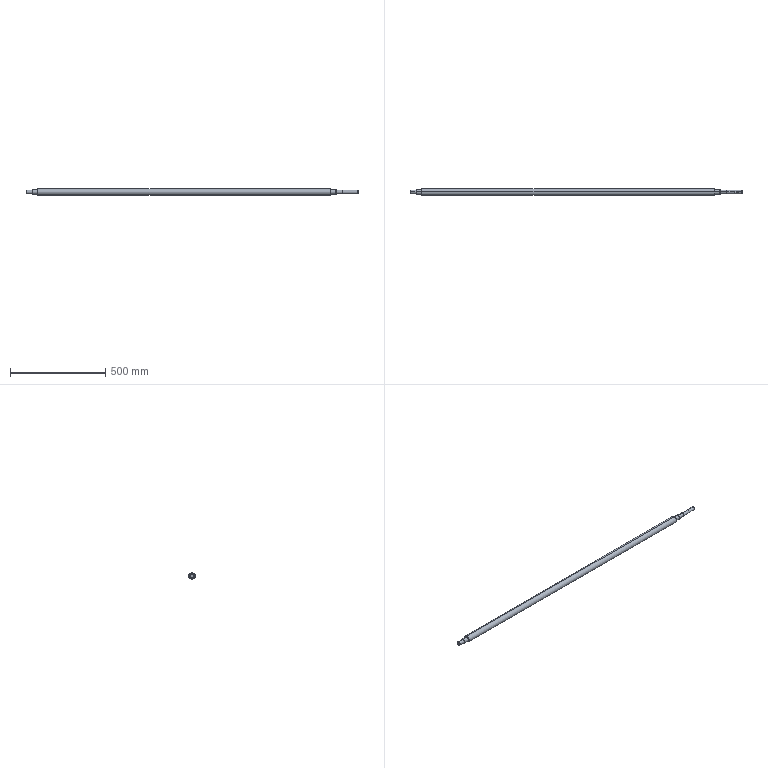Part | STEP file | Microwave Drying Flat Conveyor-CN2500x400-107-101 | 1 solid | 49 faces | box 1746 x 35 x 35 mm | volume 1552118 mm3 | cylinder 20 | cone 14 | plane 11 | torus 4 | commonest cylinder face diameters 0.4 x4 6 x4 20 x4 25 x4 18 x2 35 x2
STEP:
#1=CARTESIAN_POINT('',(-831.3,0.,9.));
#2=VERTEX_POINT('',#1);
#3=CARTESIAN_POINT('',(-831.3,0.,-9.));
#4=VERTEX_POINT('',#3);
#5=CARTESIAN_POINT('',(-831.3,0.,0.));
#6=DIRECTION('',(-1.,0.,0.));
#7=DIRECTION('',(0.,0.,-1.));
#8=AXIS2_PLACEMENT_3D('',#5,#6,#7);
#9=CIRCLE('',#8,9.);
#10=EDGE_CURVE('',#2,#4,#9,.T.);
#11=ORIENTED_EDGE('',*,*,#10,.F.);
#12=CARTESIAN_POINT('',(-830.3,0.,10.));
#13=VERTEX_POINT('',#12);
#14=CARTESIAN_POINT('',(-831.3,0.,9.));
#15=DIRECTION('',(0.7071,0.,0.7071));
#16=VECTOR('',#15,1000.);
#17=LINE('',#14,#16);
#18=EDGE_CURVE('',#2,#13,#17,.T.);
#19=ORIENTED_EDGE('',*,*,#18,.T.);
#20=CARTESIAN_POINT('',(-830.3,0.,-10.));
#21=VERTEX_POINT('',#20);
#22=CARTESIAN_POINT('',(-830.3,0.,0.));
#23=DIRECTION('',(1.,0.,0.));
#24=DIRECTION('',(0.,0.,-1.));
#25=AXIS2_PLACEMENT_3D('',#22,#23,#24);
#26=CIRCLE('',#25,10.);
#27=EDGE_CURVE('',#21,#13,#26,.T.);
#28=ORIENTED_EDGE('',*,*,#27,.F.);
#29=CARTESIAN_POINT('',(-831.3,0.,-9.));
#30=DIRECTION('',(0.7071,0.,-0.7071));
#31=VECTOR('',#30,1000.);
#32=LINE('',#29,#31);
#33=EDGE_CURVE('',#4,#21,#32,.T.);
#34=ORIENTED_EDGE('',*,*,#33,.F.);
#35=EDGE_LOOP('',(#11,#19,#28,#34));
#36=FACE_OUTER_BOUND('',#35,.T.);
#37=CARTESIAN_POINT('',(-831.3,0.,0.));
#38=DIRECTION('',(1.,0.,0.));
#39=DIRECTION('',(0.,0.,-1.));
#40=AXIS2_PLACEMENT_3D('',#37,#38,#39);
#41=CONICAL_SURFACE('',#40,9.,0.7854);
#42=ADVANCED_FACE('',(#36),#41,.T.);
#43=CARTESIAN_POINT('',(-799.3,0.,11.5));
#44=VERTEX_POINT('',#43);
#45=CARTESIAN_POINT('',(-799.3,0.,-11.5));
#46=VERTEX_POINT('',#45);
#47=CARTESIAN_POINT('',(-799.3,0.,0.));
#48=DIRECTION('',(-1.,0.,0.));
#49=DIRECTION('',(0.,0.,-1.));
#50=AXIS2_PLACEMENT_3D('',#47,#48,#49);
#51=CIRCLE('',#50,11.5);
#52=EDGE_CURVE('',#44,#46,#51,.T.);
#53=ORIENTED_EDGE('',*,*,#52,.F.);
#54=CARTESIAN_POINT('',(-798.3,0.,12.5));
#55=VERTEX_POINT('',#54);
#56=CARTESIAN_POINT('',(-799.3,0.,11.5));
#57=DIRECTION('',(0.7071,0.,0.7071));
#58=VECTOR('',#57,1000.);
#59=LINE('',#56,#58);
#60=EDGE_CURVE('',#44,#55,#59,.T.);
#61=ORIENTED_EDGE('',*,*,#60,.T.);
#62=CARTESIAN_POINT('',(-798.3,0.,-12.5));
#63=VERTEX_POINT('',#62);
#64=CARTESIAN_POINT('',(-798.3,0.,0.));
#65=DIRECTION('',(1.,0.,0.));
#66=DIRECTION('',(0.,0.,-1.));
#67=AXIS2_PLACEMENT_3D('',#64,#65,#66);
#68=CIRCLE('',#67,12.5);
#69=EDGE_CURVE('',#63,#55,#68,.T.);
#70=ORIENTED_EDGE('',*,*,#69,.F.);
#71=CARTESIAN_POINT('',(-799.3,0.,-11.5));
#72=DIRECTION('',(0.7071,0.,-0.7071));
#73=VECTOR('',#72,1000.);
#74=LINE('',#71,#73);
#75=EDGE_CURVE('',#46,#63,#74,.T.);
#76=ORIENTED_EDGE('',*,*,#75,.F.);
#77=EDGE_LOOP('',(#53,#61,#70,#76));
#78=FACE_OUTER_BOUND('',#77,.T.);
#79=CARTESIAN_POINT('',(-799.3,0.,0.));
#80=DIRECTION('',(1.,0.,0.));
#81=DIRECTION('',(0.,0.,-1.));
#82=AXIS2_PLACEMENT_3D('',#79,#80,#81);
#83=CONICAL_SURFACE('',#82,11.5,0.7854);
#84=ADVANCED_FACE('',(#78),#83,.T.);
#85=CARTESIAN_POINT('',(-771.,0.,16.5));
#86=VERTEX_POINT('',#85);
#87=CARTESIAN_POINT('',(-771.,0.,-16.5));
#88=VERTEX_POINT('',#87);
#89=CARTESIAN_POINT('',(-771.,0.,0.));
#90=DIRECTION('',(-1.,0.,0.));
#91=DIRECTION('',(0.,0.,-1.));
#92=AXIS2_PLACEMENT_3D('',#89,#90,#91);
#93=CIRCLE('',#92,16.5);
#94=EDGE_CURVE('',#86,#88,#93,.T.);
#95=ORIENTED_EDGE('',*,*,#94,.F.);
#96=CARTESIAN_POINT('',(-770.,0.,17.5));
#97=VERTEX_POINT('',#96);
#98=CARTESIAN_POINT('',(-771.,0.,16.5));
#99=DIRECTION('',(0.7071,0.,0.7071));
#100=VECTOR('',#99,1000.);
#101=LINE('',#98,#100);
#102=EDGE_CURVE('',#86,#97,#101,.T.);
#103=ORIENTED_EDGE('',*,*,#102,.T.);
#104=CARTESIAN_POINT('',(-770.,0.,-17.5));
#105=VERTEX_POINT('',#104);
#106=CARTESIAN_POINT('',(-770.,0.,0.));
#107=DIRECTION('',(1.,0.,0.));
#108=DIRECTION('',(0.,0.,-1.));
#109=AXIS2_PLACEMENT_3D('',#106,#107,#108);
#110=CIRCLE('',#109,17.5);
#111=EDGE_CURVE('',#105,#97,#110,.T.);
#112=ORIENTED_EDGE('',*,*,#111,.F.);
#113=CARTESIAN_POINT('',(-771.,0.,-16.5));
#114=DIRECTION('',(0.7071,0.,-0.7071));
#115=VECTOR('',#114,1000.);
#116=LINE('',#113,#115);
#117=EDGE_CURVE('',#88,#105,#116,.T.);
#118=ORIENTED_EDGE('',*,*,#117,.F.);
#119=EDGE_LOOP('',(#95,#103,#112,#118));
#120=FACE_OUTER_BOUND('',#119,.T.);
#121=CARTESIAN_POINT('',(-771.,0.,0.));
#122=DIRECTION('',(1.,0.,0.));
#123=DIRECTION('',(0.,0.,-1.));
#124=AXIS2_PLACEMENT_3D('',#121,#122,#123);
#125=CONICAL_SURFACE('',#124,16.5,0.7854);
#126=ADVANCED_FACE('',(#120),#125,.T.);
#127=CARTESIAN_POINT('',(771.,0.,-16.5));
#128=VERTEX_POINT('',#127);
#129=CARTESIAN_POINT('',(771.,0.,16.5));
#130=VERTEX_POINT('',#129);
#131=CARTESIAN_POINT('',(771.,0.,0.));
#132=DIRECTION('',(1.,0.,0.));
#133=DIRECTION('',(0.,0.,1.));
#134=AXIS2_PLACEMENT_3D('',#131,#132,#133);
#135=CIRCLE('',#134,16.5);
#136=EDGE_CURVE('',#128,#130,#135,.T.);
#137=ORIENTED_EDGE('',*,*,#136,.F.);
#138=CARTESIAN_POINT('',(770.,0.,-17.5));
#139=VERTEX_POINT('',#138);
#140=CARTESIAN_POINT('',(770.,0.,-17.5));
#141=DIRECTION('',(-0.7071,0.,-0.7071));
#142=VECTOR('',#141,1000.);
#143=LINE('',#140,#142);
#144=EDGE_CURVE('',#128,#139,#143,.T.);
#145=ORIENTED_EDGE('',*,*,#144,.T.);
#146=CARTESIAN_POINT('',(770.,0.,17.5));
#147=VERTEX_POINT('',#146);
#148=CARTESIAN_POINT('',(770.,0.,0.));
#149=DIRECTION('',(-1.,0.,0.));
#150=DIRECTION('',(0.,0.,1.));
#151=AXIS2_PLACEMENT_3D('',#148,#149,#150);
#152=CIRCLE('',#151,17.5);
#153=EDGE_CURVE('',#147,#139,#152,.T.);
#154=ORIENTED_EDGE('',*,*,#153,.F.);
#155=CARTESIAN_POINT('',(770.,0.,17.5));
#156=DIRECTION('',(-0.7071,0.,0.7071));
#157=VECTOR('',#156,1000.);
#158=LINE('',#155,#157);
#159=EDGE_CURVE('',#130,#147,#158,.T.);
#160=ORIENTED_EDGE('',*,*,#159,.F.);
#161=EDGE_LOOP('',(#137,#145,#154,#160));
#162=FACE_OUTER_BOUND('',#161,.T.);
#163=CARTESIAN_POINT('',(770.,0.,0.));
#164=DIRECTION('',(-1.,0.,0.));
#165=DIRECTION('',(0.,0.,1.));
#166=AXIS2_PLACEMENT_3D('',#163,#164,#165);
#167=CONICAL_SURFACE('',#166,17.5,0.7854);
#168=ADVANCED_FACE('',(#162),#167,.T.);
#169=CARTESIAN_POINT('',(799.3,0.,-11.5));
#170=VERTEX_POINT('',#169);
#171=CARTESIAN_POINT('',(799.3,0.,11.5));
#172=VERTEX_POINT('',#171);
#173=CARTESIAN_POINT('',(799.3,0.,0.));
#174=DIRECTION('',(1.,0.,0.));
#175=DIRECTION('',(0.,0.,1.));
#176=AXIS2_PLACEMENT_3D('',#173,#174,#175);
#177=CIRCLE('',#176,11.5);
#178=EDGE_CURVE('',#170,#172,#177,.T.);
#179=ORIENTED_EDGE('',*,*,#178,.F.);
#180=CARTESIAN_POINT('',(798.3,0.,-12.5));
#181=VERTEX_POINT('',#180);
#182=CARTESIAN_POINT('',(798.3,0.,-12.5));
#183=DIRECTION('',(-0.7071,0.,-0.7071));
#184=VECTOR('',#183,1000.);
#185=LINE('',#182,#184);
#186=EDGE_CURVE('',#170,#181,#185,.T.);
#187=ORIENTED_EDGE('',*,*,#186,.T.);
#188=CARTESIAN_POINT('',(798.3,0.,12.5));
#189=VERTEX_POINT('',#188);
#190=CARTESIAN_POINT('',(798.3,0.,0.));
#191=DIRECTION('',(-1.,0.,0.));
#192=DIRECTION('',(0.,0.,1.));
#193=AXIS2_PLACEMENT_3D('',#190,#191,#192);
#194=CIRCLE('',#193,12.5);
#195=EDGE_CURVE('',#189,#181,#194,.T.);
#196=ORIENTED_EDGE('',*,*,#195,.F.);
#197=CARTESIAN_POINT('',(798.3,0.,12.5));
#198=DIRECTION('',(-0.7071,0.,0.7071));
#199=VECTOR('',#198,1000.);
#200=LINE('',#197,#199);
#201=EDGE_CURVE('',#172,#189,#200,.T.);
#202=ORIENTED_EDGE('',*,*,#201,.F.);
#203=EDGE_LOOP('',(#179,#187,#196,#202));
#204=FACE_OUTER_BOUND('',#203,.T.);
#205=CARTESIAN_POINT('',(798.3,0.,0.));
#206=DIRECTION('',(-1.,0.,0.));
#207=DIRECTION('',(0.,0.,1.));
#208=AXIS2_PLACEMENT_3D('',#205,#206,#207);
#209=CONICAL_SURFACE('',#208,12.5,0.7854);
#210=ADVANCED_FACE('',(#204),#209,.T.);
#211=CARTESIAN_POINT('',(834.3,0.,9.));
#212=VERTEX_POINT('',#211);
#213=CARTESIAN_POINT('',(834.3,0.,-9.));
#214=VERTEX_POINT('',#213);
#215=CARTESIAN_POINT('',(834.3,0.,0.));
#216=DIRECTION('',(-1.,0.,0.));
#217=DIRECTION('',(0.,0.,1.));
#218=AXIS2_PLACEMENT_3D('',#215,#216,#217);
#219=CIRCLE('',#218,9.);
#220=EDGE_CURVE('',#212,#214,#219,.T.);
#221=ORIENTED_EDGE('',*,*,#220,.T.);
#222=CARTESIAN_POINT('',(833.3,0.,-10.));
#223=VERTEX_POINT('',#222);
#224=CARTESIAN_POINT('',(833.3,0.,-10.));
#225=DIRECTION('',(-0.7071,0.,-0.7071));
#226=VECTOR('',#225,1000.);
#227=LINE('',#224,#226);
#228=EDGE_CURVE('',#214,#223,#227,.T.);
#229=ORIENTED_EDGE('',*,*,#228,.T.);
#230=CARTESIAN_POINT('',(833.3,0.,10.));
#231=VERTEX_POINT('',#230);
#232=CARTESIAN_POINT('',(833.3,0.,0.));
#233=DIRECTION('',(-1.,0.,0.));
#234=DIRECTION('',(0.,0.,1.));
#235=AXIS2_PLACEMENT_3D('',#232,#233,#234);
#236=CIRCLE('',#235,10.);
#237=EDGE_CURVE('',#231,#223,#236,.T.);
#238=ORIENTED_EDGE('',*,*,#237,.F.);
#239=CARTESIAN_POINT('',(833.3,0.,10.));
#240=DIRECTION('',(-0.7071,0.,0.7071));
#241=VECTOR('',#240,1000.);
#242=LINE('',#239,#241);
#243=EDGE_CURVE('',#212,#231,#242,.T.);
#244=ORIENTED_EDGE('',*,*,#243,.F.);
#245=EDGE_LOOP('',(#221,#229,#238,#244));
#246=FACE_OUTER_BOUND('',#245,.T.);
#247=CARTESIAN_POINT('',(833.3,0.,0.));
#248=DIRECTION('',(-1.,0.,0.));
#249=DIRECTION('',(0.,0.,1.));
#250=AXIS2_PLACEMENT_3D('',#247,#248,#249);
#251=CONICAL_SURFACE('',#250,10.,0.7854);
#252=ADVANCED_FACE('',(#246),#251,.T.);
#253=CARTESIAN_POINT('',(914.3,0.,-8.));
#254=VERTEX_POINT('',#253);
#255=CARTESIAN_POINT('',(914.3,0.,8.));
#256=VERTEX_POINT('',#255);
#257=CARTESIAN_POINT('',(914.3,0.,0.));
#258=DIRECTION('',(1.,0.,0.));
#259=DIRECTION('',(0.,0.,1.));
#260=AXIS2_PLACEMENT_3D('',#257,#258,#259);
#261=CIRCLE('',#260,8.);
#262=EDGE_CURVE('',#254,#256,#261,.T.);
#263=ORIENTED_EDGE('',*,*,#262,.F.);
#264=CARTESIAN_POINT('',(913.3,0.,-9.));
#265=VERTEX_POINT('',#264);
#266=CARTESIAN_POINT('',(913.3,0.,-9.));
#267=DIRECTION('',(-0.7071,0.,-0.7071));
#268=VECTOR('',#267,1000.);
#269=LINE('',#266,#268);
#270=EDGE_CURVE('',#254,#265,#269,.T.);
#271=ORIENTED_EDGE('',*,*,#270,.T.);
#272=CARTESIAN_POINT('',(913.3,0.,9.));
#273=VERTEX_POINT('',#272);
#274=CARTESIAN_POINT('',(913.3,0.,0.));
#275=DIRECTION('',(-1.,0.,0.));
#276=DIRECTION('',(0.,0.,1.));
#277=AXIS2_PLACEMENT_3D('',#274,#275,#276);
#278=CIRCLE('',#277,9.);
#279=EDGE_CURVE('',#273,#265,#278,.T.);
#280=ORIENTED_EDGE('',*,*,#279,.F.);
#281=CARTESIAN_POINT('',(913.3,0.,9.));
#282=DIRECTION('',(-0.7071,0.,0.7071));
#283=VECTOR('',#282,1000.);
#284=LINE('',#281,#283);
#285=EDGE_CURVE('',#256,#273,#284,.T.);
#286=ORIENTED_EDGE('',*,*,#285,.F.);
#287=EDGE_LOOP('',(#263,#271,#280,#286));
#288=FACE_OUTER_BOUND('',#287,.T.);
#289=CARTESIAN_POINT('',(913.3,0.,0.));
#290=DIRECTION('',(-1.,0.,0.));
#291=DIRECTION('',(0.,0.,1.));
#292=AXIS2_PLACEMENT_3D('',#289,#290,#291);
#293=CONICAL_SURFACE('',#292,9.,0.7854);
#294=ADVANCED_FACE('',(#288),#293,.T.);
#295=CARTESIAN_POINT('',(-799.3,0.,10.));
#296=VERTEX_POINT('',#295);
#297=CARTESIAN_POINT('',(-799.3,0.,-10.));
#298=VERTEX_POINT('',#297);
#299=CARTESIAN_POINT('',(-799.3,0.,0.));
#300=DIRECTION('',(-1.,0.,0.));
#301=DIRECTION('',(0.,0.,1.));
#302=AXIS2_PLACEMENT_3D('',#299,#300,#301);
#303=CIRCLE('',#302,10.);
#304=EDGE_CURVE('',#296,#298,#303,.T.);
#305=ORIENTED_EDGE('',*,*,#304,.T.);
#306=CARTESIAN_POINT('',(-727.8,0.,-10.));
#307=DIRECTION('',(-1.,0.,0.));
#308=VECTOR('',#307,1000.);
#309=LINE('',#306,#308);
#310=EDGE_CURVE('',#298,#21,#309,.T.);
#311=ORIENTED_EDGE('',*,*,#310,.T.);
#312=ORIENTED_EDGE('',*,*,#27,.T.);
#313=CARTESIAN_POINT('',(-727.8,0.,10.));
#314=DIRECTION('',(-1.,0.,0.));
#315=VECTOR('',#314,1000.);
#316=LINE('',#313,#315);
#317=EDGE_CURVE('',#296,#13,#316,.T.);
#318=ORIENTED_EDGE('',*,*,#317,.F.);
#319=EDGE_LOOP('',(#305,#311,#312,#318));
#320=FACE_OUTER_BOUND('',#319,.T.);
#321=CARTESIAN_POINT('',(-727.8,0.,0.));
#322=DIRECTION('',(-1.,0.,0.));
#323=DIRECTION('',(0.,0.,1.));
#324=AXIS2_PLACEMENT_3D('',#321,#322,#323);
#325=CYLINDRICAL_SURFACE('',#324,10.);
#326=ADVANCED_FACE('',(#320),#325,.T.);
#327=CARTESIAN_POINT('',(-771.,0.,12.5));
#328=VERTEX_POINT('',#327);
#329=CARTESIAN_POINT('',(-771.,0.,-12.5));
#330=VERTEX_POINT('',#329);
#331=CARTESIAN_POINT('',(-771.,0.,0.));
#332=DIRECTION('',(-1.,0.,0.));
#333=DIRECTION('',(0.,0.,1.));
#334=AXIS2_PLACEMENT_3D('',#331,#332,#333);
#335=CIRCLE('',#334,12.5);
#336=EDGE_CURVE('',#328,#330,#335,.T.);
#337=ORIENTED_EDGE('',*,*,#336,.T.);
#338=CARTESIAN_POINT('',(-727.8,0.,-12.5));
#339=DIRECTION('',(-1.,0.,0.));
#340=VECTOR('',#339,1000.);
#341=LINE('',#338,#340);
#342=EDGE_CURVE('',#330,#63,#341,.T.);
#343=ORIENTED_EDGE('',*,*,#342,.T.);
#344=ORIENTED_EDGE('',*,*,#69,.T.);
#345=CARTESIAN_POINT('',(-727.8,0.,12.5));
#346=DIRECTION('',(-1.,0.,0.));
#347=VECTOR('',#346,1000.);
#348=LINE('',#345,#347);
#349=EDGE_CURVE('',#328,#55,#348,.T.);
#350=ORIENTED_EDGE('',*,*,#349,.F.);
#351=EDGE_LOOP('',(#337,#343,#344,#350));
#352=FACE_OUTER_BOUND('',#351,.T.);
#353=CARTESIAN_POINT('',(-727.8,0.,0.));
#354=DIRECTION('',(-1.,0.,0.));
#355=DIRECTION('',(0.,0.,1.));
#356=AXIS2_PLACEMENT_3D('',#353,#354,#355);
#357=CYLINDRICAL_SURFACE('',#356,12.5);
#358=ADVANCED_FACE('',(#352),#357,.T.);
#359=ORIENTED_EDGE('',*,*,#153,.T.);
#360=CARTESIAN_POINT('',(-727.8,0.,-17.5));
#361=DIRECTION('',(-1.,0.,0.));
#362=VECTOR('',#361,1000.);
#363=LINE('',#360,#362);
#364=EDGE_CURVE('',#139,#105,#363,.T.);
#365=ORIENTED_EDGE('',*,*,#364,.T.);
#366=ORIENTED_EDGE('',*,*,#111,.T.);
#367=CARTESIAN_POINT('',(-727.8,0.,17.5));
#368=DIRECTION('',(-1.,0.,0.));
#369=VECTOR('',#368,1000.);
#370=LINE('',#367,#369);
#371=EDGE_CURVE('',#147,#97,#370,.T.);
#372=ORIENTED_EDGE('',*,*,#371,.F.);
#373=EDGE_LOOP('',(#359,#365,#366,#372));
#374=FACE_OUTER_BOUND('',#373,.T.);
#375=CARTESIAN_POINT('',(-727.8,0.,0.));
#376=DIRECTION('',(-1.,0.,0.));
#377=DIRECTION('',(0.,0.,1.));
#378=AXIS2_PLACEMENT_3D('',#375,#376,#377);
#379=CYLINDRICAL_SURFACE('',#378,17.5);
#380=ADVANCED_FACE('',(#374),#379,.T.);
#381=ORIENTED_EDGE('',*,*,#195,.T.);
#382=CARTESIAN_POINT('',(771.,0.,-12.5));
#383=VERTEX_POINT('',#382);
#384=CARTESIAN_POINT('',(-727.8,0.,-12.5));
#385=DIRECTION('',(-1.,0.,0.));
#386=VECTOR('',#385,1000.);
#387=LINE('',#384,#386);
#388=EDGE_CURVE('',#181,#383,#387,.T.);
#389=ORIENTED_EDGE('',*,*,#388,.T.);
#390=CARTESIAN_POINT('',(771.,0.,12.5));
#391=VERTEX_POINT('',#390);
#392=CARTESIAN_POINT('',(771.,0.,0.));
#393=DIRECTION('',(-1.,0.,0.));
#394=DIRECTION('',(0.,0.,1.));
#395=AXIS2_PLACEMENT_3D('',#392,#393,#394);
#396=CIRCLE('',#395,12.5);
#397=EDGE_CURVE('',#391,#383,#396,.T.);
#398=ORIENTED_EDGE('',*,*,#397,.F.);
#399=CARTESIAN_POINT('',(-727.8,0.,12.5));
#400=DIRECTION('',(-1.,0.,0.));
#401=VECTOR('',#400,1000.);
#402=LINE('',#399,#401);
#403=EDGE_CURVE('',#189,#391,#402,.T.);
#404=ORIENTED_EDGE('',*,*,#403,.F.);
#405=EDGE_LOOP('',(#381,#389,#398,#404));
#406=FACE_OUTER_BOUND('',#405,.T.);
#407=CARTESIAN_POINT('',(-727.8,0.,0.));
#408=DIRECTION('',(-1.,0.,0.));
#409=DIRECTION('',(0.,0.,1.));
#410=AXIS2_PLACEMENT_3D('',#407,#408,#409);
#411=CYLINDRICAL_SURFACE('',#410,12.5);
#412=ADVANCED_FACE('',(#406),#411,.T.);
#413=ORIENTED_EDGE('',*,*,#237,.T.);
#414=CARTESIAN_POINT('',(799.3,0.,-10.));
#415=VERTEX_POINT('',#414);
#416=CARTESIAN_POINT('',(-727.8,0.,-10.));
#417=DIRECTION('',(-1.,0.,0.));
#418=VECTOR('',#417,1000.);
#419=LINE('',#416,#418);
#420=EDGE_CURVE('',#223,#415,#419,.T.);
#421=ORIENTED_EDGE('',*,*,#420,.T.);
#422=CARTESIAN_POINT('',(799.3,0.,10.));
#423=VERTEX_POINT('',#422);
#424=CARTESIAN_POINT('',(799.3,0.,0.));
#425=DIRECTION('',(-1.,0.,0.));
#426=DIRECTION('',(0.,0.,1.));
#427=AXIS2_PLACEMENT_3D('',#424,#425,#426);
#428=CIRCLE('',#427,10.);
#429=EDGE_CURVE('',#423,#415,#428,.T.);
#430=ORIENTED_EDGE('',*,*,#429,.F.);
#431=CARTESIAN_POINT('',(-727.8,0.,10.));
#432=DIRECTION('',(-1.,0.,0.));
#433=VECTOR('',#432,1000.);
#434=LINE('',#431,#433);
#435=EDGE_CURVE('',#231,#423,#434,.T.);
#436=ORIENTED_EDGE('',*,*,#435,.F.);
#437=EDGE_LOOP('',(#413,#421,#430,#436));
#438=FACE_OUTER_BOUND('',#437,.T.);
#439=CARTESIAN_POINT('',(-727.8,0.,0.));
#440=DIRECTION('',(-1.,0.,0.));
#441=DIRECTION('',(0.,0.,1.));
#442=AXIS2_PLACEMENT_3D('',#439,#440,#441);
#443=CYLINDRICAL_SURFACE('',#442,10.);
#444=ADVANCED_FACE('',(#438),#443,.T.);
#445=ORIENTED_EDGE('',*,*,#279,.T.);
#446=CARTESIAN_POINT('',(-727.8,0.,-9.));
#447=DIRECTION('',(-1.,0.,0.));
#448=VECTOR('',#447,1000.);
#449=LINE('',#446,#448);
#450=EDGE_CURVE('',#265,#214,#449,.T.);
#451=ORIENTED_EDGE('',*,*,#450,.T.);
#452=ORIENTED_EDGE('',*,*,#220,.F.);
#453=CARTESIAN_POINT('',(874.3,0.,9.));
#454=VERTEX_POINT('',#453);
#455=CARTESIAN_POINT('',(-727.8,0.,9.));
#456=DIRECTION('',(-1.,0.,0.));
#457=VECTOR('',#456,1000.);
#458=LINE('',#455,#457);
#459=EDGE_CURVE('',#454,#212,#458,.T.);
#460=ORIENTED_EDGE('',*,*,#459,.F.);
#461=CARTESIAN_POINT('',(877.3,3.,8.485));
#462=VERTEX_POINT('',#461);
#463=CARTESIAN_POINT('',(874.3,0.,9.));
#464=CARTESIAN_POINT('',(874.3,0.1996,9.));
#465=CARTESIAN_POINT('',(874.32,0.3957,8.993));
#466=CARTESIAN_POINT('',(874.397,0.7809,8.968));
#467=CARTESIAN_POINT('',(874.455,0.9721,8.949));
#468=CARTESIAN_POINT('',(874.606,1.335,8.902));
#469=CARTESIAN_POINT('',(874.698,1.506,8.875));
#470=CARTESIAN_POINT('',(874.916,1.831,8.813));
#471=CARTESIAN_POINT('',(875.041,1.984,8.78));
#472=CARTESIAN_POINT('',(875.453,2.396,8.68));
#473=CARTESIAN_POINT('',(875.785,2.618,8.612));
#474=CARTESIAN_POINT('',(876.325,2.844,8.539));
#475=CARTESIAN_POINT('',(876.515,2.902,8.519));
#476=CARTESIAN_POINT('',(876.903,2.98,8.492));
#477=CARTESIAN_POINT('',(877.1,3.,8.485));
#478=CARTESIAN_POINT('',(877.3,3.,8.485));
#479=B_SPLINE_CURVE_WITH_KNOTS('',3,(#463,#464,#465,#466,#467,#468,#469,#470,#471,#472,#473,#474,#475,#476,#477,#478),.UNSPECIFIED.,.F.,.F.,(4,2,2,2,2,2,2,4),(0.,0.0005901,0.00118,0.00177,0.00236,0.003541,0.004131,0.004721),.UNSPECIFIED.);
#480=EDGE_CURVE('',#454,#462,#479,.T.);
#481=ORIENTED_EDGE('',*,*,#480,.T.);
#482=CARTESIAN_POINT('',(891.3,3.,8.485));
#483=VERTEX_POINT('',#482);
#484=CARTESIAN_POINT('',(-727.8,3.,8.485));
#485=DIRECTION('',(1.,0.,0.));
#486=VECTOR('',#485,1000.);
#487=LINE('',#484,#486);
#488=EDGE_CURVE('',#462,#483,#487,.T.);
#489=ORIENTED_EDGE('',*,*,#488,.T.);
#490=CARTESIAN_POINT('',(894.3,0.,9.));
#491=VERTEX_POINT('',#490);
#492=CARTESIAN_POINT('',(891.3,3.,8.485));
#493=CARTESIAN_POINT('',(891.5,3.,8.485));
#494=CARTESIAN_POINT('',(891.696,2.98,8.492));
#495=CARTESIAN_POINT('',(892.081,2.903,8.519));
#496=CARTESIAN_POINT('',(892.272,2.845,8.539));
#497=CARTESIAN_POINT('',(892.634,2.694,8.588));
#498=CARTESIAN_POINT('',(892.806,2.602,8.616));
#499=CARTESIAN_POINT('',(893.131,2.385,8.679));
#500=CARTESIAN_POINT('',(893.283,2.259,8.713));
#501=CARTESIAN_POINT('',(893.695,1.848,8.813));
#502=CARTESIAN_POINT('',(893.918,1.516,8.879));
#503=CARTESIAN_POINT('',(894.144,0.9753,8.949));
#504=CARTESIAN_POINT('',(894.202,0.7852,8.968));
#505=CARTESIAN_POINT('',(894.28,0.3966,8.993));
#506=CARTESIAN_POINT('',(894.3,0.1996,9.));
#507=CARTESIAN_POINT('',(894.3,0.,9.));
#508=B_SPLINE_CURVE_WITH_KNOTS('',3,(#492,#493,#494,#495,#496,#497,#498,#499,#500,#501,#502,#503,#504,#505,#506,#507),.UNSPECIFIED.,.F.,.F.,(4,2,2,2,2,2,2,4),(0.,0.0005901,0.00118,0.00177,0.00236,0.00354,0.00413,0.004721),.UNSPECIFIED.);
#509=EDGE_CURVE('',#483,#491,#508,.T.);
#510=ORIENTED_EDGE('',*,*,#509,.T.);
#511=CARTESIAN_POINT('',(-727.8,0.,9.));
#512=DIRECTION('',(-1.,0.,0.));
#513=VECTOR('',#512,1000.);
#514=LINE('',#511,#513);
#515=EDGE_CURVE('',#273,#491,#514,.T.);
#516=ORIENTED_EDGE('',*,*,#515,.F.);
#517=EDGE_LOOP('',(#445,#451,#452,#460,#481,#489,#510,#516));
#518=FACE_OUTER_BOUND('',#517,.T.);
#519=CARTESIAN_POINT('',(-727.8,0.,0.));
#520=DIRECTION('',(-1.,0.,0.));
#521=DIRECTION('',(0.,0.,1.));
#522=AXIS2_PLACEMENT_3D('',#519,#520,#521);
#523=CYLINDRICAL_SURFACE('',#522,9.);
#524=ADVANCED_FACE('',(#518),#523,.T.);
#525=CARTESIAN_POINT('',(-831.3,0.,0.));
#526=DIRECTION('',(-1.,0.,0.));
#527=DIRECTION('',(0.,0.,-1.));
#528=AXIS2_PLACEMENT_3D('',#525,#526,#527);
#529=CIRCLE('',#528,9.);
#530=EDGE_CURVE('',#4,#2,#529,.T.);
#531=ORIENTED_EDGE('',*,*,#530,.T.);
#532=ORIENTED_EDGE('',*,*,#10,.T.);
#533=EDGE_LOOP('',(#531,#532));
#534=FACE_OUTER_BOUND('',#533,.T.);
#535=CARTESIAN_POINT('',(-831.3,0.,-10.));
#536=DIRECTION('',(1.,0.,0.));
#537=DIRECTION('',(0.,0.,-1.));
#538=AXIS2_PLACEMENT_3D('',#535,#536,#537);
#539=PLANE('',#538);
#540=ADVANCED_FACE('',(#534),#539,.F.);
#541=CARTESIAN_POINT('',(914.3,0.,0.));
#542=DIRECTION('',(1.,0.,0.));
#543=DIRECTION('',(0.,0.,1.));
#544=AXIS2_PLACEMENT_3D('',#541,#542,#543);
#545=CIRCLE('',#544,8.);
#546=EDGE_CURVE('',#256,#254,#545,.T.);
#547=ORIENTED_EDGE('',*,*,#546,.T.);
#548=ORIENTED_EDGE('',*,*,#262,.T.);
#549=EDGE_LOOP('',(#547,#548));
#550=FACE_OUTER_BOUND('',#549,.T.);
#551=CARTESIAN_POINT('',(914.3,0.,0.));
#552=DIRECTION('',(-1.,0.,0.));
#553=DIRECTION('',(0.,0.,1.));
#554=AXIS2_PLACEMENT_3D('',#551,#552,#553);
#555=PLANE('',#554);
#556=ADVANCED_FACE('',(#550),#555,.F.);
#557=ORIENTED_EDGE('',*,*,#450,.F.);
#558=CARTESIAN_POINT('',(913.3,0.,0.));
#559=DIRECTION('',(-1.,0.,0.));
#560=DIRECTION('',(0.,0.,1.));
#561=AXIS2_PLACEMENT_3D('',#558,#559,#560);
#562=CIRCLE('',#561,9.);
#563=EDGE_CURVE('',#265,#273,#562,.T.);
#564=ORIENTED_EDGE('',*,*,#563,.T.);
#565=ORIENTED_EDGE('',*,*,#515,.T.);
#566=CARTESIAN_POINT('',(894.3,-0.04707,9.));
#567=VERTEX_POINT('',#566);
#568=CARTESIAN_POINT('',(894.3,0.,0.));
#569=DIRECTION('',(1.,0.,0.));
#570=DIRECTION('',(0.,0.,-1.));
#571=AXIS2_PLACEMENT_3D('',#568,#569,#570);
#572=CIRCLE('',#571,9.);
#573=EDGE_CURVE('',#491,#567,#572,.T.);
#574=ORIENTED_EDGE('',*,*,#573,.T.);
#575=CARTESIAN_POINT('',(891.3,-3.047,8.468));
#576=VERTEX_POINT('',#575);
#577=CARTESIAN_POINT('',(894.3,-0.04707,9.));
#578=CARTESIAN_POINT('',(894.3,-0.2468,8.999));
#579=CARTESIAN_POINT('',(894.28,-0.4428,8.991));
#580=CARTESIAN_POINT('',(894.203,-0.8281,8.964));
#581=CARTESIAN_POINT('',(894.145,-1.019,8.944));
#582=CARTESIAN_POINT('',(893.994,-1.382,8.895));
#583=CARTESIAN_POINT('',(893.902,-1.553,8.866));
#584=CARTESIAN_POINT('',(893.684,-1.878,8.803));
#585=CARTESIAN_POINT('',(893.559,-2.031,8.769));
#586=CARTESIAN_POINT('',(893.147,-2.443,8.667));
#587=CARTESIAN_POINT('',(892.816,-2.665,8.598));
#588=CARTESIAN_POINT('',(892.275,-2.891,8.523));
#589=CARTESIAN_POINT('',(892.085,-2.949,8.503));
#590=CARTESIAN_POINT('',(891.697,-3.027,8.476));
#591=CARTESIAN_POINT('',(891.5,-3.047,8.468));
#592=CARTESIAN_POINT('',(891.3,-3.047,8.468));
#593=B_SPLINE_CURVE_WITH_KNOTS('',3,(#577,#578,#579,#580,#581,#582,#583,#584,#585,#586,#587,#588,#589,#590,#591,#592),.UNSPECIFIED.,.F.,.F.,(4,2,2,2,2,2,2,4),(0.,0.0005903,0.001181,0.001771,0.002361,0.003542,0.004132,0.004723),.UNSPECIFIED.);
#594=EDGE_CURVE('',#567,#576,#593,.T.);
#595=ORIENTED_EDGE('',*,*,#594,.T.);
#596=CARTESIAN_POINT('',(877.3,-3.047,8.468));
#597=VERTEX_POINT('',#596);
#598=CARTESIAN_POINT('',(-727.8,-3.047,8.468));
#599=DIRECTION('',(-1.,0.,0.));
#600=VECTOR('',#599,1000.);
#601=LINE('',#598,#600);
#602=EDGE_CURVE('',#576,#597,#601,.T.);
#603=ORIENTED_EDGE('',*,*,#602,.T.);
#604=CARTESIAN_POINT('',(874.3,-0.04707,9.));
#605=VERTEX_POINT('',#604);
#606=CARTESIAN_POINT('',(877.3,-3.047,8.468));
#607=CARTESIAN_POINT('',(877.1,-3.047,8.468));
#608=CARTESIAN_POINT('',(876.904,-3.027,8.476));
#609=CARTESIAN_POINT('',(876.519,-2.95,8.503));
#610=CARTESIAN_POINT('',(876.328,-2.892,8.523));
#611=CARTESIAN_POINT('',(875.965,-2.741,8.573));
#612=CARTESIAN_POINT('',(875.794,-2.649,8.602));
#613=CARTESIAN_POINT('',(875.469,-2.431,8.666));
#614=CARTESIAN_POINT('',(875.316,-2.306,8.701));
#615=CARTESIAN_POINT('',(874.905,-1.895,8.803));
#616=CARTESIAN_POINT('',(874.682,-1.563,8.871));
#617=CARTESIAN_POINT('',(874.456,-1.023,8.944));
#618=CARTESIAN_POINT('',(874.398,-0.8324,8.964));
#619=CARTESIAN_POINT('',(874.32,-0.4437,8.991));
#620=CARTESIAN_POINT('',(874.3,-0.2468,8.999));
#621=CARTESIAN_POINT('',(874.3,-0.04707,9.));
#622=B_SPLINE_CURVE_WITH_KNOTS('',3,(#606,#607,#608,#609,#610,#611,#612,#613,#614,#615,#616,#617,#618,#619,#620,#621),.UNSPECIFIED.,.F.,.F.,(4,2,2,2,2,2,2,4),(0.,0.0005903,0.001181,0.001771,0.002361,0.003542,0.004132,0.004722),.UNSPECIFIED.);
#623=EDGE_CURVE('',#597,#605,#622,.T.);
#624=ORIENTED_EDGE('',*,*,#623,.T.);
#625=CARTESIAN_POINT('',(874.3,0.,0.));
#626=DIRECTION('',(-1.,0.,0.));
#627=DIRECTION('',(0.,0.,1.));
#628=AXIS2_PLACEMENT_3D('',#625,#626,#627);
#629=CIRCLE('',#628,9.);
#630=EDGE_CURVE('',#605,#454,#629,.T.);
#631=ORIENTED_EDGE('',*,*,#630,.T.);
#632=ORIENTED_EDGE('',*,*,#459,.T.);
#633=CARTESIAN_POINT('',(834.3,0.,0.));
#634=DIRECTION('',(-1.,0.,0.));
#635=DIRECTION('',(0.,0.,1.));
#636=AXIS2_PLACEMENT_3D('',#633,#634,#635);
#637=CIRCLE('',#636,9.);
#638=EDGE_CURVE('',#214,#212,#637,.T.);
#639=ORIENTED_EDGE('',*,*,#638,.F.);
#640=EDGE_LOOP('',(#557,#564,#565,#574,#595,#603,#624,#631,#632,#639));
#641=FACE_OUTER_BOUND('',#640,.T.);
#642=CARTESIAN_POINT('',(-727.8,0.,0.));
#643=DIRECTION('',(-1.,0.,0.));
#644=DIRECTION('',(0.,0.,1.));
#645=AXIS2_PLACEMENT_3D('',#642,#643,#644);
#646=CYLINDRICAL_SURFACE('',#645,9.);
#647=ADVANCED_FACE('',(#641),#646,.T.);
#648=ORIENTED_EDGE('',*,*,#420,.F.);
#649=CARTESIAN_POINT('',(833.3,0.,0.));
#650=DIRECTION('',(-1.,0.,0.));
#651=DIRECTION('',(0.,0.,1.));
#652=AXIS2_PLACEMENT_3D('',#649,#650,#651);
#653=CIRCLE('',#652,10.);
#654=EDGE_CURVE('',#223,#231,#653,.T.);
#655=ORIENTED_EDGE('',*,*,#654,.T.);
#656=ORIENTED_EDGE('',*,*,#435,.T.);
#657=CARTESIAN_POINT('',(799.3,0.,0.));
#658=DIRECTION('',(-1.,0.,0.));
#659=DIRECTION('',(0.,0.,1.));
#660=AXIS2_PLACEMENT_3D('',#657,#658,#659);
#661=CIRCLE('',#660,10.);
#662=EDGE_CURVE('',#415,#423,#661,.T.);
#663=ORIENTED_EDGE('',*,*,#662,.F.);
#664=EDGE_LOOP('',(#648,#655,#656,#663));
#665=FACE_OUTER_BOUND('',#664,.T.);
#666=CARTESIAN_POINT('',(-727.8,0.,0.));
#667=DIRECTION('',(-1.,0.,0.));
#668=DIRECTION('',(0.,0.,1.));
#669=AXIS2_PLACEMENT_3D('',#666,#667,#668);
#670=CYLINDRICAL_SURFACE('',#669,10.);
#671=ADVANCED_FACE('',(#665),#670,.T.);
#672=CARTESIAN_POINT('',(799.3,0.,0.));
#673=DIRECTION('',(1.,0.,0.));
#674=DIRECTION('',(0.,0.,1.));
#675=AXIS2_PLACEMENT_3D('',#672,#673,#674);
#676=CIRCLE('',#675,11.5);
#677=EDGE_CURVE('',#172,#170,#676,.T.);
#678=ORIENTED_EDGE('',*,*,#677,.T.);
#679=ORIENTED_EDGE('',*,*,#178,.T.);
#680=EDGE_LOOP('',(#678,#679));
#681=FACE_OUTER_BOUND('',#680,.T.);
#682=ORIENTED_EDGE('',*,*,#429,.T.);
#683=ORIENTED_EDGE('',*,*,#662,.T.);
#684=EDGE_LOOP('',(#682,#683));
#685=FACE_BOUND('',#684,.T.);
#686=CARTESIAN_POINT('',(799.3,0.,-12.5));
#687=DIRECTION('',(-1.,0.,0.));
#688=DIRECTION('',(0.,0.,1.));
#689=AXIS2_PLACEMENT_3D('',#686,#687,#688);
#690=PLANE('',#689);
#691=ADVANCED_FACE('',(#681,#685),#690,.F.);
#692=ORIENTED_EDGE('',*,*,#388,.F.);
#693=CARTESIAN_POINT('',(798.3,0.,0.));
#694=DIRECTION('',(-1.,0.,0.));
#695=DIRECTION('',(0.,0.,1.));
#696=AXIS2_PLACEMENT_3D('',#693,#694,#695);
#697=CIRCLE('',#696,12.5);
#698=EDGE_CURVE('',#181,#189,#697,.T.);
#699=ORIENTED_EDGE('',*,*,#698,.T.);
#700=ORIENTED_EDGE('',*,*,#403,.T.);
#701=CARTESIAN_POINT('',(771.,0.,0.));
#702=DIRECTION('',(-1.,0.,0.));
#703=DIRECTION('',(0.,0.,1.));
#704=AXIS2_PLACEMENT_3D('',#701,#702,#703);
#705=CIRCLE('',#704,12.5);
#706=EDGE_CURVE('',#383,#391,#705,.T.);
#707=ORIENTED_EDGE('',*,*,#706,.F.);
#708=EDGE_LOOP('',(#692,#699,#700,#707));
#709=FACE_OUTER_BOUND('',#708,.T.);
#710=CARTESIAN_POINT('',(-727.8,0.,0.));
#711=DIRECTION('',(-1.,0.,0.));
#712=DIRECTION('',(0.,0.,1.));
#713=AXIS2_PLACEMENT_3D('',#710,#711,#712);
#714=CYLINDRICAL_SURFACE('',#713,12.5);
#715=ADVANCED_FACE('',(#709),#714,.T.);
#716=CARTESIAN_POINT('',(771.,0.,0.));
#717=DIRECTION('',(1.,0.,0.));
#718=DIRECTION('',(0.,0.,1.));
#719=AXIS2_PLACEMENT_3D('',#716,#717,#718);
#720=CIRCLE('',#719,16.5);
#721=EDGE_CURVE('',#130,#128,#720,.T.);
#722=ORIENTED_EDGE('',*,*,#721,.T.);
#723=ORIENTED_EDGE('',*,*,#136,.T.);
#724=EDGE_LOOP('',(#722,#723));
#725=FACE_OUTER_BOUND('',#724,.T.);
#726=ORIENTED_EDGE('',*,*,#397,.T.);
#727=ORIENTED_EDGE('',*,*,#706,.T.);
#728=EDGE_LOOP('',(#726,#727));
#729=FACE_BOUND('',#728,.T.);
#730=CARTESIAN_POINT('',(771.,0.,-12.5));
#731=DIRECTION('',(-1.,0.,0.));
#732=DIRECTION('',(0.,0.,1.));
#733=AXIS2_PLACEMENT_3D('',#730,#731,#732);
#734=PLANE('',#733);
#735=ADVANCED_FACE('',(#725,#729),#734,.F.);
#736=ORIENTED_EDGE('',*,*,#364,.F.);
#737=CARTESIAN_POINT('',(770.,0.,0.));
#738=DIRECTION('',(-1.,0.,0.));
#739=DIRECTION('',(0.,0.,1.));
#740=AXIS2_PLACEMENT_3D('',#737,#738,#739);
#741=CIRCLE('',#740,17.5);
#742=EDGE_CURVE('',#139,#147,#741,.T.);
#743=ORIENTED_EDGE('',*,*,#742,.T.);
#744=ORIENTED_EDGE('',*,*,#371,.T.);
#745=CARTESIAN_POINT('',(-770.,0.,0.));
#746=DIRECTION('',(1.,0.,0.));
#747=DIRECTION('',(0.,0.,-1.));
#748=AXIS2_PLACEMENT_3D('',#745,#746,#747);
#749=CIRCLE('',#748,17.5);
#750=EDGE_CURVE('',#97,#105,#749,.T.);
#751=ORIENTED_EDGE('',*,*,#750,.T.);
#752=EDGE_LOOP('',(#736,#743,#744,#751));
#753=FACE_OUTER_BOUND('',#752,.T.);
#754=CARTESIAN_POINT('',(-727.8,0.,0.));
#755=DIRECTION('',(-1.,0.,0.));
#756=DIRECTION('',(0.,0.,1.));
#757=AXIS2_PLACEMENT_3D('',#754,#755,#756);
#758=CYLINDRICAL_SURFACE('',#757,17.5);
#759=ADVANCED_FACE('',(#753),#758,.T.);
#760=CARTESIAN_POINT('',(-771.,0.,0.));
#761=DIRECTION('',(-1.,0.,0.));
#762=DIRECTION('',(0.,0.,-1.));
#763=AXIS2_PLACEMENT_3D('',#760,#761,#762);
#764=CIRCLE('',#763,16.5);
#765=EDGE_CURVE('',#88,#86,#764,.T.);
#766=ORIENTED_EDGE('',*,*,#765,.T.);
#767=ORIENTED_EDGE('',*,*,#94,.T.);
#768=EDGE_LOOP('',(#766,#767));
#769=FACE_OUTER_BOUND('',#768,.T.);
#770=ORIENTED_EDGE('',*,*,#336,.F.);
#771=CARTESIAN_POINT('',(-771.,0.,0.));
#772=DIRECTION('',(-1.,0.,0.));
#773=DIRECTION('',(0.,0.,1.));
#774=AXIS2_PLACEMENT_3D('',#771,#772,#773);
#775=CIRCLE('',#774,12.5);
#776=EDGE_CURVE('',#330,#328,#775,.T.);
#777=ORIENTED_EDGE('',*,*,#776,.F.);
#778=EDGE_LOOP('',(#770,#777));
#779=FACE_BOUND('',#778,.T.);
#780=CARTESIAN_POINT('',(-771.,0.,-17.5));
#781=DIRECTION('',(1.,0.,0.));
#782=DIRECTION('',(0.,0.,-1.));
#783=AXIS2_PLACEMENT_3D('',#780,#781,#782);
#784=PLANE('',#783);
#785=ADVANCED_FACE('',(#769,#779),#784,.F.);
#786=ORIENTED_EDGE('',*,*,#342,.F.);
#787=ORIENTED_EDGE('',*,*,#776,.T.);
#788=ORIENTED_EDGE('',*,*,#349,.T.);
#789=CARTESIAN_POINT('',(-798.3,0.,0.));
#790=DIRECTION('',(1.,0.,0.));
#791=DIRECTION('',(0.,0.,-1.));
#792=AXIS2_PLACEMENT_3D('',#789,#790,#791);
#793=CIRCLE('',#792,12.5);
#794=EDGE_CURVE('',#55,#63,#793,.T.);
#795=ORIENTED_EDGE('',*,*,#794,.T.);
#796=EDGE_LOOP('',(#786,#787,#788,#795));
#797=FACE_OUTER_BOUND('',#796,.T.);
#798=CARTESIAN_POINT('',(-727.8,0.,0.));
#799=DIRECTION('',(-1.,0.,0.));
#800=DIRECTION('',(0.,0.,1.));
#801=AXIS2_PLACEMENT_3D('',#798,#799,#800);
#802=CYLINDRICAL_SURFACE('',#801,12.5);
#803=ADVANCED_FACE('',(#797),#802,.T.);
#804=CARTESIAN_POINT('',(-799.3,0.,0.));
#805=DIRECTION('',(-1.,0.,0.));
#806=DIRECTION('',(0.,0.,-1.));
#807=AXIS2_PLACEMENT_3D('',#804,#805,#806);
#808=CIRCLE('',#807,11.5);
#809=EDGE_CURVE('',#46,#44,#808,.T.);
#810=ORIENTED_EDGE('',*,*,#809,.T.);
#811=ORIENTED_EDGE('',*,*,#52,.T.);
#812=EDGE_LOOP('',(#810,#811));
#813=FACE_OUTER_BOUND('',#812,.T.);
#814=ORIENTED_EDGE('',*,*,#304,.F.);
#815=CARTESIAN_POINT('',(-799.3,0.,0.));
#816=DIRECTION('',(-1.,0.,0.));
#817=DIRECTION('',(0.,0.,1.));
#818=AXIS2_PLACEMENT_3D('',#815,#816,#817);
#819=CIRCLE('',#818,10.);
#820=EDGE_CURVE('',#298,#296,#819,.T.);
#821=ORIENTED_EDGE('',*,*,#820,.F.);
#822=EDGE_LOOP('',(#814,#821));
#823=FACE_BOUND('',#822,.T.);
#824=CARTESIAN_POINT('',(-799.3,0.,-12.5));
#825=DIRECTION('',(1.,0.,0.));
#826=DIRECTION('',(0.,0.,-1.));
#827=AXIS2_PLACEMENT_3D('',#824,#825,#826);
#828=PLANE('',#827);
#829=ADVANCED_FACE('',(#813,#823),#828,.F.);
#830=ORIENTED_EDGE('',*,*,#310,.F.);
#831=ORIENTED_EDGE('',*,*,#820,.T.);
#832=ORIENTED_EDGE('',*,*,#317,.T.);
#833=CARTESIAN_POINT('',(-830.3,0.,0.));
#834=DIRECTION('',(1.,0.,0.));
#835=DIRECTION('',(0.,0.,-1.));
#836=AXIS2_PLACEMENT_3D('',#833,#834,#835);
#837=CIRCLE('',#836,10.);
#838=EDGE_CURVE('',#13,#21,#837,.T.);
#839=ORIENTED_EDGE('',*,*,#838,.T.);
#840=EDGE_LOOP('',(#830,#831,#832,#839));
#841=FACE_OUTER_BOUND('',#840,.T.);
#842=CARTESIAN_POINT('',(-727.8,0.,0.));
#843=DIRECTION('',(-1.,0.,0.));
#844=DIRECTION('',(0.,0.,1.));
#845=AXIS2_PLACEMENT_3D('',#842,#843,#844);
#846=CYLINDRICAL_SURFACE('',#845,10.);
#847=ADVANCED_FACE('',(#841),#846,.T.);
#848=CARTESIAN_POINT('',(877.3,-3.047,5.7));
#849=VERTEX_POINT('',#848);
#850=CARTESIAN_POINT('',(877.3,-3.047,5.5));
#851=DIRECTION('',(0.,0.,1.));
#852=VECTOR('',#851,1000.);
#853=LINE('',#850,#852);
#854=EDGE_CURVE('',#849,#597,#853,.T.);
#855=ORIENTED_EDGE('',*,*,#854,.F.);
#856=CARTESIAN_POINT('',(874.3,-0.04707,5.7));
#857=VERTEX_POINT('',#856);
#858=CARTESIAN_POINT('',(877.3,-0.04707,5.7));
#859=DIRECTION('',(0.,0.,-1.));
#860=DIRECTION('',(-1.,0.,0.));
#861=AXIS2_PLACEMENT_3D('',#858,#859,#860);
#862=CIRCLE('',#861,3.);
#863=EDGE_CURVE('',#849,#857,#862,.T.);
#864=ORIENTED_EDGE('',*,*,#863,.T.);
#865=CARTESIAN_POINT('',(874.3,-0.04707,5.5));
#866=DIRECTION('',(0.,0.,1.));
#867=VECTOR('',#866,1000.);
#868=LINE('',#865,#867);
#869=EDGE_CURVE('',#857,#605,#868,.T.);
#870=ORIENTED_EDGE('',*,*,#869,.T.);
#871=ORIENTED_EDGE('',*,*,#623,.F.);
#872=EDGE_LOOP('',(#855,#864,#870,#871));
#873=FACE_OUTER_BOUND('',#872,.T.);
#874=CARTESIAN_POINT('',(877.3,-0.04707,5.5));
#875=DIRECTION('',(0.,0.,1.));
#876=DIRECTION('',(1.,0.,0.));
#877=AXIS2_PLACEMENT_3D('',#874,#875,#876);
#878=CYLINDRICAL_SURFACE('',#877,3.);
#879=ADVANCED_FACE('',(#873),#878,.F.);
#880=ORIENTED_EDGE('',*,*,#869,.F.);
#881=CARTESIAN_POINT('',(874.3,0.,5.7));
#882=VERTEX_POINT('',#881);
#883=CARTESIAN_POINT('',(874.3,0.,5.7));
#884=DIRECTION('',(0.,1.,0.));
#885=VECTOR('',#884,1000.);
#886=LINE('',#883,#885);
#887=EDGE_CURVE('',#857,#882,#886,.T.);
#888=ORIENTED_EDGE('',*,*,#887,.T.);
#889=CARTESIAN_POINT('',(874.3,0.,5.5));
#890=DIRECTION('',(0.,0.,1.));
#891=VECTOR('',#890,1000.);
#892=LINE('',#889,#891);
#893=EDGE_CURVE('',#882,#454,#892,.T.);
#894=ORIENTED_EDGE('',*,*,#893,.T.);
#895=ORIENTED_EDGE('',*,*,#630,.F.);
#896=EDGE_LOOP('',(#880,#888,#894,#895));
#897=FACE_OUTER_BOUND('',#896,.T.);
#898=CARTESIAN_POINT('',(874.3,0.,5.5));
#899=DIRECTION('',(-1.,0.,0.));
#900=DIRECTION('',(0.,0.,1.));
#901=AXIS2_PLACEMENT_3D('',#898,#899,#900);
#902=PLANE('',#901);
#903=ADVANCED_FACE('',(#897),#902,.F.);
#904=ORIENTED_EDGE('',*,*,#893,.F.);
#905=CARTESIAN_POINT('',(877.3,3.,5.7));
#906=VERTEX_POINT('',#905);
#907=CARTESIAN_POINT('',(877.3,0.,5.7));
#908=DIRECTION('',(0.,0.,-1.));
#909=DIRECTION('',(-1.,0.,0.));
#910=AXIS2_PLACEMENT_3D('',#907,#908,#909);
#911=CIRCLE('',#910,3.);
#912=EDGE_CURVE('',#882,#906,#911,.T.);
#913=ORIENTED_EDGE('',*,*,#912,.T.);
#914=CARTESIAN_POINT('',(877.3,3.,5.5));
#915=DIRECTION('',(0.,0.,1.));
#916=VECTOR('',#915,1000.);
#917=LINE('',#914,#916);
#918=EDGE_CURVE('',#906,#462,#917,.T.);
#919=ORIENTED_EDGE('',*,*,#918,.T.);
#920=ORIENTED_EDGE('',*,*,#480,.F.);
#921=EDGE_LOOP('',(#904,#913,#919,#920));
#922=FACE_OUTER_BOUND('',#921,.T.);
#923=CARTESIAN_POINT('',(877.3,0.,5.5));
#924=DIRECTION('',(0.,0.,1.));
#925=DIRECTION('',(1.,0.,0.));
#926=AXIS2_PLACEMENT_3D('',#923,#924,#925);
#927=CYLINDRICAL_SURFACE('',#926,3.);
#928=ADVANCED_FACE('',(#922),#927,.F.);
#929=ORIENTED_EDGE('',*,*,#918,.F.);
#930=CARTESIAN_POINT('',(891.3,3.,5.7));
#931=VERTEX_POINT('',#930);
#932=CARTESIAN_POINT('',(891.3,3.,5.7));
#933=DIRECTION('',(1.,0.,0.));
#934=VECTOR('',#933,1000.);
#935=LINE('',#932,#934);
#936=EDGE_CURVE('',#906,#931,#935,.T.);
#937=ORIENTED_EDGE('',*,*,#936,.T.);
#938=CARTESIAN_POINT('',(891.3,3.,5.5));
#939=DIRECTION('',(0.,0.,1.));
#940=VECTOR('',#939,1000.);
#941=LINE('',#938,#940);
#942=EDGE_CURVE('',#931,#483,#941,.T.);
#943=ORIENTED_EDGE('',*,*,#942,.T.);
#944=ORIENTED_EDGE('',*,*,#488,.F.);
#945=EDGE_LOOP('',(#929,#937,#943,#944));
#946=FACE_OUTER_BOUND('',#945,.T.);
#947=CARTESIAN_POINT('',(891.3,3.,5.5));
#948=DIRECTION('',(0.,1.,0.));
#949=DIRECTION('',(-1.,0.,0.));
#950=AXIS2_PLACEMENT_3D('',#947,#948,#949);
#951=PLANE('',#950);
#952=ADVANCED_FACE('',(#946),#951,.F.);
#953=ORIENTED_EDGE('',*,*,#942,.F.);
#954=CARTESIAN_POINT('',(894.3,0.,5.7));
#955=VERTEX_POINT('',#954);
#956=CARTESIAN_POINT('',(891.3,0.,5.7));
#957=DIRECTION('',(0.,0.,-1.));
#958=DIRECTION('',(-1.,0.,0.));
#959=AXIS2_PLACEMENT_3D('',#956,#957,#958);
#960=CIRCLE('',#959,3.);
#961=EDGE_CURVE('',#931,#955,#960,.T.);
#962=ORIENTED_EDGE('',*,*,#961,.T.);
#963=CARTESIAN_POINT('',(894.3,0.,5.5));
#964=DIRECTION('',(0.,0.,1.));
#965=VECTOR('',#964,1000.);
#966=LINE('',#963,#965);
#967=EDGE_CURVE('',#955,#491,#966,.T.);
#968=ORIENTED_EDGE('',*,*,#967,.T.);
#969=ORIENTED_EDGE('',*,*,#509,.F.);
#970=EDGE_LOOP('',(#953,#962,#968,#969));
#971=FACE_OUTER_BOUND('',#970,.T.);
#972=CARTESIAN_POINT('',(891.3,0.,5.5));
#973=DIRECTION('',(0.,0.,1.));
#974=DIRECTION('',(1.,0.,0.));
#975=AXIS2_PLACEMENT_3D('',#972,#973,#974);
#976=CYLINDRICAL_SURFACE('',#975,3.);
#977=ADVANCED_FACE('',(#971),#976,.F.);
#978=ORIENTED_EDGE('',*,*,#967,.F.);
#979=CARTESIAN_POINT('',(894.3,-0.04707,5.7));
#980=VERTEX_POINT('',#979);
#981=CARTESIAN_POINT('',(894.3,-0.04707,5.7));
#982=DIRECTION('',(0.,-1.,0.));
#983=VECTOR('',#982,1000.);
#984=LINE('',#981,#983);
#985=EDGE_CURVE('',#955,#980,#984,.T.);
#986=ORIENTED_EDGE('',*,*,#985,.T.);
#987=CARTESIAN_POINT('',(894.3,-0.04707,5.5));
#988=DIRECTION('',(0.,0.,1.));
#989=VECTOR('',#988,1000.);
#990=LINE('',#987,#989);
#991=EDGE_CURVE('',#980,#567,#990,.T.);
#992=ORIENTED_EDGE('',*,*,#991,.T.);
#993=ORIENTED_EDGE('',*,*,#573,.F.);
#994=EDGE_LOOP('',(#978,#986,#992,#993));
#995=FACE_OUTER_BOUND('',#994,.T.);
#996=CARTESIAN_POINT('',(894.3,0.,5.5));
#997=DIRECTION('',(1.,0.,0.));
#998=DIRECTION('',(0.,0.,-1.));
#999=AXIS2_PLACEMENT_3D('',#996,#997,#998);
#1000=PLANE('',#999);
#1001=ADVANCED_FACE('',(#995),#1000,.F.);
#1002=ORIENTED_EDGE('',*,*,#991,.F.);
#1003=CARTESIAN_POINT('',(891.3,-3.047,5.7));
#1004=VERTEX_POINT('',#1003);
#1005=CARTESIAN_POINT('',(891.3,-0.04707,5.7));
#1006=DIRECTION('',(0.,0.,-1.));
#1007=DIRECTION('',(-1.,0.,0.));
#1008=AXIS2_PLACEMENT_3D('',#1005,#1006,#1007);
#1009=CIRCLE('',#1008,3.);
#1010=EDGE_CURVE('',#980,#1004,#1009,.T.);
#1011=ORIENTED_EDGE('',*,*,#1010,.T.);
#1012=CARTESIAN_POINT('',(891.3,-3.047,5.5));
#1013=DIRECTION('',(0.,0.,1.));
#1014=VECTOR('',#1013,1000.);
#1015=LINE('',#1012,#1014);
#1016=EDGE_CURVE('',#1004,#576,#1015,.T.);
#1017=ORIENTED_EDGE('',*,*,#1016,.T.);
#1018=ORIENTED_EDGE('',*,*,#594,.F.);
#1019=EDGE_LOOP('',(#1002,#1011,#1017,#1018));
#1020=FACE_OUTER_BOUND('',#1019,.T.);
#1021=CARTESIAN_POINT('',(891.3,-0.04707,5.5));
#1022=DIRECTION('',(0.,0.,1.));
#1023=DIRECTION('',(1.,0.,0.));
#1024=AXIS2_PLACEMENT_3D('',#1021,#1022,#1023);
#1025=CYLINDRICAL_SURFACE('',#1024,3.);
#1026=ADVANCED_FACE('',(#1020),#1025,.F.);
#1027=ORIENTED_EDGE('',*,*,#1016,.F.);
#1028=CARTESIAN_POINT('',(877.3,-3.047,5.7));
#1029=DIRECTION('',(-1.,0.,0.));
#1030=VECTOR('',#1029,1000.);
#1031=LINE('',#1028,#1030);
#1032=EDGE_CURVE('',#1004,#849,#1031,.T.);
#1033=ORIENTED_EDGE('',*,*,#1032,.T.);
#1034=ORIENTED_EDGE('',*,*,#854,.T.);
#1035=ORIENTED_EDGE('',*,*,#602,.F.);
#1036=EDGE_LOOP('',(#1027,#1033,#1034,#1035));
#1037=FACE_OUTER_BOUND('',#1036,.T.);
#1038=CARTESIAN_POINT('',(891.3,-3.047,5.5));
#1039=DIRECTION('',(0.,-1.,0.));
#1040=DIRECTION('',(1.,0.,0.));
#1041=AXIS2_PLACEMENT_3D('',#1038,#1039,#1040);
#1042=PLANE('',#1041);
#1043=ADVANCED_FACE('',(#1037),#1042,.F.);
#1044=CARTESIAN_POINT('',(894.1,-0.04707,5.5));
#1045=VERTEX_POINT('',#1044);
#1046=CARTESIAN_POINT('',(894.1,0.,5.5));
#1047=VERTEX_POINT('',#1046);
#1048=CARTESIAN_POINT('',(894.1,0.,5.5));
#1049=DIRECTION('',(0.,1.,0.));
#1050=VECTOR('',#1049,1000.);
#1051=LINE('',#1048,#1050);
#1052=EDGE_CURVE('',#1045,#1047,#1051,.T.);
#1053=ORIENTED_EDGE('',*,*,#1052,.T.);
#1054=CARTESIAN_POINT('',(891.3,2.8,5.5));
#1055=VERTEX_POINT('',#1054);
#1056=CARTESIAN_POINT('',(891.3,0.,5.5));
#1057=DIRECTION('',(0.,0.,1.));
#1058=DIRECTION('',(-1.,0.,0.));
#1059=AXIS2_PLACEMENT_3D('',#1056,#1057,#1058);
#1060=CIRCLE('',#1059,2.8);
#1061=EDGE_CURVE('',#1047,#1055,#1060,.T.);
#1062=ORIENTED_EDGE('',*,*,#1061,.T.);
#1063=CARTESIAN_POINT('',(877.3,2.8,5.5));
#1064=VERTEX_POINT('',#1063);
#1065=CARTESIAN_POINT('',(877.3,2.8,5.5));
#1066=DIRECTION('',(-1.,0.,0.));
#1067=VECTOR('',#1066,1000.);
#1068=LINE('',#1065,#1067);
#1069=EDGE_CURVE('',#1055,#1064,#1068,.T.);
#1070=ORIENTED_EDGE('',*,*,#1069,.T.);
#1071=CARTESIAN_POINT('',(874.5,0.,5.5));
#1072=VERTEX_POINT('',#1071);
#1073=CARTESIAN_POINT('',(877.3,0.,5.5));
#1074=DIRECTION('',(0.,0.,1.));
#1075=DIRECTION('',(-1.,0.,0.));
#1076=AXIS2_PLACEMENT_3D('',#1073,#1074,#1075);
#1077=CIRCLE('',#1076,2.8);
#1078=EDGE_CURVE('',#1064,#1072,#1077,.T.);
#1079=ORIENTED_EDGE('',*,*,#1078,.T.);
#1080=CARTESIAN_POINT('',(874.5,-0.04707,5.5));
#1081=VERTEX_POINT('',#1080);
#1082=CARTESIAN_POINT('',(874.5,-0.04707,5.5));
#1083=DIRECTION('',(0.,-1.,0.));
#1084=VECTOR('',#1083,1000.);
#1085=LINE('',#1082,#1084);
#1086=EDGE_CURVE('',#1072,#1081,#1085,.T.);
#1087=ORIENTED_EDGE('',*,*,#1086,.T.);
#1088=CARTESIAN_POINT('',(877.3,-2.847,5.5));
#1089=VERTEX_POINT('',#1088);
#1090=CARTESIAN_POINT('',(877.3,-0.04707,5.5));
#1091=DIRECTION('',(0.,0.,1.));
#1092=DIRECTION('',(-1.,0.,0.));
#1093=AXIS2_PLACEMENT_3D('',#1090,#1091,#1092);
#1094=CIRCLE('',#1093,2.8);
#1095=EDGE_CURVE('',#1081,#1089,#1094,.T.);
#1096=ORIENTED_EDGE('',*,*,#1095,.T.);
#1097=CARTESIAN_POINT('',(891.3,-2.847,5.5));
#1098=VERTEX_POINT('',#1097);
#1099=CARTESIAN_POINT('',(891.3,-2.847,5.5));
#1100=DIRECTION('',(1.,0.,0.));
#1101=VECTOR('',#1100,1000.);
#1102=LINE('',#1099,#1101);
#1103=EDGE_CURVE('',#1089,#1098,#1102,.T.);
#1104=ORIENTED_EDGE('',*,*,#1103,.T.);
#1105=CARTESIAN_POINT('',(891.3,-0.04707,5.5));
#1106=DIRECTION('',(0.,0.,1.));
#1107=DIRECTION('',(-1.,0.,0.));
#1108=AXIS2_PLACEMENT_3D('',#1105,#1106,#1107);
#1109=CIRCLE('',#1108,2.8);
#1110=EDGE_CURVE('',#1098,#1045,#1109,.T.);
#1111=ORIENTED_EDGE('',*,*,#1110,.T.);
#1112=EDGE_LOOP('',(#1053,#1062,#1070,#1079,#1087,#1096,#1104,#1111));
#1113=FACE_OUTER_BOUND('',#1112,.T.);
#1114=CARTESIAN_POINT('',(877.3,-0.04707,5.5));
#1115=DIRECTION('',(0.,0.,-1.));
#1116=DIRECTION('',(-1.,0.,0.));
#1117=AXIS2_PLACEMENT_3D('',#1114,#1115,#1116);
#1118=PLANE('',#1117);
#1119=ADVANCED_FACE('',(#1113),#1118,.F.);
#1120=CARTESIAN_POINT('',(874.5,-0.04707,5.7));
#1121=DIRECTION('',(0.,-1.,0.));
#1122=DIRECTION('',(1.,0.,0.));
#1123=AXIS2_PLACEMENT_3D('',#1120,#1121,#1122);
#1124=CIRCLE('',#1123,0.2);
#1125=EDGE_CURVE('',#857,#1081,#1124,.T.);
#1126=ORIENTED_EDGE('',*,*,#1125,.F.);
#1127=ORIENTED_EDGE('',*,*,#863,.F.);
#1128=CARTESIAN_POINT('',(877.3,-2.847,5.7));
#1129=DIRECTION('',(-1.,0.,0.));
#1130=DIRECTION('',(0.,0.,1.));
#1131=AXIS2_PLACEMENT_3D('',#1128,#1129,#1130);
#1132=CIRCLE('',#1131,0.2);
#1133=EDGE_CURVE('',#1089,#849,#1132,.T.);
#1134=ORIENTED_EDGE('',*,*,#1133,.F.);
#1135=ORIENTED_EDGE('',*,*,#1095,.F.);
#1136=EDGE_LOOP('',(#1126,#1127,#1134,#1135));
#1137=FACE_OUTER_BOUND('',#1136,.T.);
#1138=CARTESIAN_POINT('',(877.3,-0.04707,5.7));
#1139=DIRECTION('',(0.,0.,-1.));
#1140=DIRECTION('',(-1.,0.,0.));
#1141=AXIS2_PLACEMENT_3D('',#1138,#1139,#1140);
#1142=TOROIDAL_SURFACE('',#1141,2.8,0.2);
#1143=ADVANCED_FACE('',(#1137),#1142,.F.);
#1144=ORIENTED_EDGE('',*,*,#1133,.T.);
#1145=ORIENTED_EDGE('',*,*,#1032,.F.);
#1146=CARTESIAN_POINT('',(891.3,-2.847,5.7));
#1147=DIRECTION('',(-1.,0.,0.));
#1148=DIRECTION('',(0.,0.,1.));
#1149=AXIS2_PLACEMENT_3D('',#1146,#1147,#1148);
#1150=CIRCLE('',#1149,0.2);
#1151=EDGE_CURVE('',#1098,#1004,#1150,.T.);
#1152=ORIENTED_EDGE('',*,*,#1151,.F.);
#1153=ORIENTED_EDGE('',*,*,#1103,.F.);
#1154=EDGE_LOOP('',(#1144,#1145,#1152,#1153));
#1155=FACE_OUTER_BOUND('',#1154,.T.);
#1156=CARTESIAN_POINT('',(877.3,-2.847,5.7));
#1157=DIRECTION('',(-1.,0.,0.));
#1158=DIRECTION('',(0.,-1.,0.));
#1159=AXIS2_PLACEMENT_3D('',#1156,#1157,#1158);
#1160=CYLINDRICAL_SURFACE('',#1159,0.2);
#1161=ADVANCED_FACE('',(#1155),#1160,.F.);
#1162=ORIENTED_EDGE('',*,*,#1125,.T.);
#1163=ORIENTED_EDGE('',*,*,#1086,.F.);
#1164=CARTESIAN_POINT('',(874.5,0.,5.7));
#1165=DIRECTION('',(0.,-1.,0.));
#1166=DIRECTION('',(0.,0.,-1.));
#1167=AXIS2_PLACEMENT_3D('',#1164,#1165,#1166);
#1168=CIRCLE('',#1167,0.2);
#1169=EDGE_CURVE('',#882,#1072,#1168,.T.);
#1170=ORIENTED_EDGE('',*,*,#1169,.F.);
#1171=ORIENTED_EDGE('',*,*,#887,.F.);
#1172=EDGE_LOOP('',(#1162,#1163,#1170,#1171));
#1173=FACE_OUTER_BOUND('',#1172,.T.);
#1174=CARTESIAN_POINT('',(874.5,-0.04707,5.7));
#1175=DIRECTION('',(0.,1.,0.));
#1176=DIRECTION('',(0.,0.,1.));
#1177=AXIS2_PLACEMENT_3D('',#1174,#1175,#1176);
#1178=CYLINDRICAL_SURFACE('',#1177,0.2);
#1179=ADVANCED_FACE('',(#1173),#1178,.F.);
#1180=ORIENTED_EDGE('',*,*,#1151,.T.);
#1181=ORIENTED_EDGE('',*,*,#1010,.F.);
#1182=CARTESIAN_POINT('',(894.1,-0.04707,5.7));
#1183=DIRECTION('',(0.,-1.,0.));
#1184=DIRECTION('',(0.,0.,-1.));
#1185=AXIS2_PLACEMENT_3D('',#1182,#1183,#1184);
#1186=CIRCLE('',#1185,0.2);
#1187=EDGE_CURVE('',#1045,#980,#1186,.T.);
#1188=ORIENTED_EDGE('',*,*,#1187,.F.);
#1189=ORIENTED_EDGE('',*,*,#1110,.F.);
#1190=EDGE_LOOP('',(#1180,#1181,#1188,#1189));
#1191=FACE_OUTER_BOUND('',#1190,.T.);
#1192=CARTESIAN_POINT('',(891.3,-0.04707,5.7));
#1193=DIRECTION('',(0.,0.,-1.));
#1194=DIRECTION('',(-1.,0.,0.));
#1195=AXIS2_PLACEMENT_3D('',#1192,#1193,#1194);
#1196=TOROIDAL_SURFACE('',#1195,2.8,0.2);
#1197=ADVANCED_FACE('',(#1191),#1196,.F.);
#1198=ORIENTED_EDGE('',*,*,#1169,.T.);
#1199=ORIENTED_EDGE('',*,*,#1078,.F.);
#1200=CARTESIAN_POINT('',(877.3,2.8,5.7));
#1201=DIRECTION('',(-1.,0.,0.));
#1202=DIRECTION('',(0.,0.,1.));
#1203=AXIS2_PLACEMENT_3D('',#1200,#1201,#1202);
#1204=CIRCLE('',#1203,0.2);
#1205=EDGE_CURVE('',#906,#1064,#1204,.T.);
#1206=ORIENTED_EDGE('',*,*,#1205,.F.);
#1207=ORIENTED_EDGE('',*,*,#912,.F.);
#1208=EDGE_LOOP('',(#1198,#1199,#1206,#1207));
#1209=FACE_OUTER_BOUND('',#1208,.T.);
#1210=CARTESIAN_POINT('',(877.3,0.,5.7));
#1211=DIRECTION('',(0.,0.,-1.));
#1212=DIRECTION('',(-1.,0.,0.));
#1213=AXIS2_PLACEMENT_3D('',#1210,#1211,#1212);
#1214=TOROIDAL_SURFACE('',#1213,2.8,0.2);
#1215=ADVANCED_FACE('',(#1209),#1214,.F.);
#1216=ORIENTED_EDGE('',*,*,#1187,.T.);
#1217=ORIENTED_EDGE('',*,*,#985,.F.);
#1218=CARTESIAN_POINT('',(894.1,0.,5.7));
#1219=DIRECTION('',(0.,-1.,0.));
#1220=DIRECTION('',(1.,0.,0.));
#1221=AXIS2_PLACEMENT_3D('',#1218,#1219,#1220);
#1222=CIRCLE('',#1221,0.2);
#1223=EDGE_CURVE('',#1047,#955,#1222,.T.);
#1224=ORIENTED_EDGE('',*,*,#1223,.F.);
#1225=ORIENTED_EDGE('',*,*,#1052,.F.);
#1226=EDGE_LOOP('',(#1216,#1217,#1224,#1225));
#1227=FACE_OUTER_BOUND('',#1226,.T.);
#1228=CARTESIAN_POINT('',(894.1,-0.04707,5.7));
#1229=DIRECTION('',(0.,-1.,0.));
#1230=DIRECTION('',(0.,0.,-1.));
#1231=AXIS2_PLACEMENT_3D('',#1228,#1229,#1230);
#1232=CYLINDRICAL_SURFACE('',#1231,0.2);
#1233=ADVANCED_FACE('',(#1227),#1232,.F.);
#1234=ORIENTED_EDGE('',*,*,#1205,.T.);
#1235=ORIENTED_EDGE('',*,*,#1069,.F.);
#1236=CARTESIAN_POINT('',(891.3,2.8,5.7));
#1237=DIRECTION('',(-1.,0.,0.));
#1238=DIRECTION('',(0.,0.,1.));
#1239=AXIS2_PLACEMENT_3D('',#1236,#1237,#1238);
#1240=CIRCLE('',#1239,0.2);
#1241=EDGE_CURVE('',#931,#1055,#1240,.T.);
#1242=ORIENTED_EDGE('',*,*,#1241,.F.);
#1243=ORIENTED_EDGE('',*,*,#936,.F.);
#1244=EDGE_LOOP('',(#1234,#1235,#1242,#1243));
#1245=FACE_OUTER_BOUND('',#1244,.T.);
#1246=CARTESIAN_POINT('',(877.3,2.8,5.7));
#1247=DIRECTION('',(1.,0.,0.));
#1248=DIRECTION('',(0.,1.,0.));
#1249=AXIS2_PLACEMENT_3D('',#1246,#1247,#1248);
#1250=CYLINDRICAL_SURFACE('',#1249,0.2);
#1251=ADVANCED_FACE('',(#1245),#1250,.F.);
#1252=ORIENTED_EDGE('',*,*,#1223,.T.);
#1253=ORIENTED_EDGE('',*,*,#961,.F.);
#1254=ORIENTED_EDGE('',*,*,#1241,.T.);
#1255=ORIENTED_EDGE('',*,*,#1061,.F.);
#1256=EDGE_LOOP('',(#1252,#1253,#1254,#1255));
#1257=FACE_OUTER_BOUND('',#1256,.T.);
#1258=CARTESIAN_POINT('',(891.3,0.,5.7));
#1259=DIRECTION('',(0.,0.,-1.));
#1260=DIRECTION('',(-1.,0.,0.));
#1261=AXIS2_PLACEMENT_3D('',#1258,#1259,#1260);
#1262=TOROIDAL_SURFACE('',#1261,2.8,0.2);
#1263=ADVANCED_FACE('',(#1257),#1262,.F.);
#1264=ORIENTED_EDGE('',*,*,#270,.F.);
#1265=ORIENTED_EDGE('',*,*,#546,.F.);
#1266=ORIENTED_EDGE('',*,*,#285,.T.);
#1267=ORIENTED_EDGE('',*,*,#563,.F.);
#1268=EDGE_LOOP('',(#1264,#1265,#1266,#1267));
#1269=FACE_OUTER_BOUND('',#1268,.T.);
#1270=CARTESIAN_POINT('',(913.3,0.,0.));
#1271=DIRECTION('',(-1.,0.,0.));
#1272=DIRECTION('',(0.,0.,1.));
#1273=AXIS2_PLACEMENT_3D('',#1270,#1271,#1272);
#1274=CONICAL_SURFACE('',#1273,9.,0.7854);
#1275=ADVANCED_FACE('',(#1269),#1274,.T.);
#1276=ORIENTED_EDGE('',*,*,#228,.F.);
#1277=ORIENTED_EDGE('',*,*,#638,.T.);
#1278=ORIENTED_EDGE('',*,*,#243,.T.);
#1279=ORIENTED_EDGE('',*,*,#654,.F.);
#1280=EDGE_LOOP('',(#1276,#1277,#1278,#1279));
#1281=FACE_OUTER_BOUND('',#1280,.T.);
#1282=CARTESIAN_POINT('',(833.3,0.,0.));
#1283=DIRECTION('',(-1.,0.,0.));
#1284=DIRECTION('',(0.,0.,1.));
#1285=AXIS2_PLACEMENT_3D('',#1282,#1283,#1284);
#1286=CONICAL_SURFACE('',#1285,10.,0.7854);
#1287=ADVANCED_FACE('',(#1281),#1286,.T.);
#1288=ORIENTED_EDGE('',*,*,#186,.F.);
#1289=ORIENTED_EDGE('',*,*,#677,.F.);
#1290=ORIENTED_EDGE('',*,*,#201,.T.);
#1291=ORIENTED_EDGE('',*,*,#698,.F.);
#1292=EDGE_LOOP('',(#1288,#1289,#1290,#1291));
#1293=FACE_OUTER_BOUND('',#1292,.T.);
#1294=CARTESIAN_POINT('',(798.3,0.,0.));
#1295=DIRECTION('',(-1.,0.,0.));
#1296=DIRECTION('',(0.,0.,1.));
#1297=AXIS2_PLACEMENT_3D('',#1294,#1295,#1296);
#1298=CONICAL_SURFACE('',#1297,12.5,0.7854);
#1299=ADVANCED_FACE('',(#1293),#1298,.T.);
#1300=ORIENTED_EDGE('',*,*,#144,.F.);
#1301=ORIENTED_EDGE('',*,*,#721,.F.);
#1302=ORIENTED_EDGE('',*,*,#159,.T.);
#1303=ORIENTED_EDGE('',*,*,#742,.F.);
#1304=EDGE_LOOP('',(#1300,#1301,#1302,#1303));
#1305=FACE_OUTER_BOUND('',#1304,.T.);
#1306=CARTESIAN_POINT('',(770.,0.,0.));
#1307=DIRECTION('',(-1.,0.,0.));
#1308=DIRECTION('',(0.,0.,1.));
#1309=AXIS2_PLACEMENT_3D('',#1306,#1307,#1308);
#1310=CONICAL_SURFACE('',#1309,17.5,0.7854);
#1311=ADVANCED_FACE('',(#1305),#1310,.T.);
#1312=ORIENTED_EDGE('',*,*,#102,.F.);
#1313=ORIENTED_EDGE('',*,*,#765,.F.);
#1314=ORIENTED_EDGE('',*,*,#117,.T.);
#1315=ORIENTED_EDGE('',*,*,#750,.F.);
#1316=EDGE_LOOP('',(#1312,#1313,#1314,#1315));
#1317=FACE_OUTER_BOUND('',#1316,.T.);
#1318=CARTESIAN_POINT('',(-771.,0.,0.));
#1319=DIRECTION('',(1.,0.,0.));
#1320=DIRECTION('',(0.,0.,-1.));
#1321=AXIS2_PLACEMENT_3D('',#1318,#1319,#1320);
#1322=CONICAL_SURFACE('',#1321,16.5,0.7854);
#1323=ADVANCED_FACE('',(#1317),#1322,.T.);
#1324=ORIENTED_EDGE('',*,*,#60,.F.);
#1325=ORIENTED_EDGE('',*,*,#809,.F.);
#1326=ORIENTED_EDGE('',*,*,#75,.T.);
#1327=ORIENTED_EDGE('',*,*,#794,.F.);
#1328=EDGE_LOOP('',(#1324,#1325,#1326,#1327));
#1329=FACE_OUTER_BOUND('',#1328,.T.);
#1330=CARTESIAN_POINT('',(-799.3,0.,0.));
#1331=DIRECTION('',(1.,0.,0.));
#1332=DIRECTION('',(0.,0.,-1.));
#1333=AXIS2_PLACEMENT_3D('',#1330,#1331,#1332);
#1334=CONICAL_SURFACE('',#1333,11.5,0.7854);
#1335=ADVANCED_FACE('',(#1329),#1334,.T.);
#1336=ORIENTED_EDGE('',*,*,#18,.F.);
#1337=ORIENTED_EDGE('',*,*,#530,.F.);
#1338=ORIENTED_EDGE('',*,*,#33,.T.);
#1339=ORIENTED_EDGE('',*,*,#838,.F.);
#1340=EDGE_LOOP('',(#1336,#1337,#1338,#1339));
#1341=FACE_OUTER_BOUND('',#1340,.T.);
#1342=CARTESIAN_POINT('',(-831.3,0.,0.));
#1343=DIRECTION('',(1.,0.,0.));
#1344=DIRECTION('',(0.,0.,-1.));
#1345=AXIS2_PLACEMENT_3D('',#1342,#1343,#1344);
#1346=CONICAL_SURFACE('',#1345,9.,0.7854);
#1347=ADVANCED_FACE('',(#1341),#1346,.T.);
#1348=CLOSED_SHELL('',(#42,#84,#126,#168,#210,#252,#294,#326,#358,#380,#412,#444,#524,#540,#556,#647,#671,#691,#715,#735,#759,#785,#803,#829,#847,#879,#903,#928,#952,#977,#1001,#1026,#1043,#1119,#1143,#1161,#1179,#1197,#1215,#1233,#1251,#1263,#1275,#1287,#1299,#1311,#1323,#1335,#1347));
#1349=MANIFOLD_SOLID_BREP('',#1348);
#1350=CARTESIAN_POINT('',(0.,0.,0.));
#1351=DIRECTION('',(0.,0.,1.));
#1352=DIRECTION('',(1.,0.,0.));
#1353=AXIS2_PLACEMENT_3D('',#1350,#1351,#1352);
#1354=(LENGTH_UNIT()NAMED_UNIT(*)SI_UNIT(.MILLI.,.METRE.));
#1355=UNCERTAINTY_MEASURE_WITH_UNIT(LENGTH_MEASURE(0.00001),#1354,'','');
#1356=(NAMED_UNIT(*)PLANE_ANGLE_UNIT()SI_UNIT($,.RADIAN.));
#1357=(NAMED_UNIT(*)SI_UNIT($,.STERADIAN.)SOLID_ANGLE_UNIT());
#1358=(GEOMETRIC_REPRESENTATION_CONTEXT(3)GLOBAL_UNCERTAINTY_ASSIGNED_CONTEXT((#1355))GLOBAL_UNIT_ASSIGNED_CONTEXT((#1354,#1356,#1357))REPRESENTATION_CONTEXT('',''));
#1359=ADVANCED_BREP_SHAPE_REPRESENTATION('',(#1349,#1353),#1358);